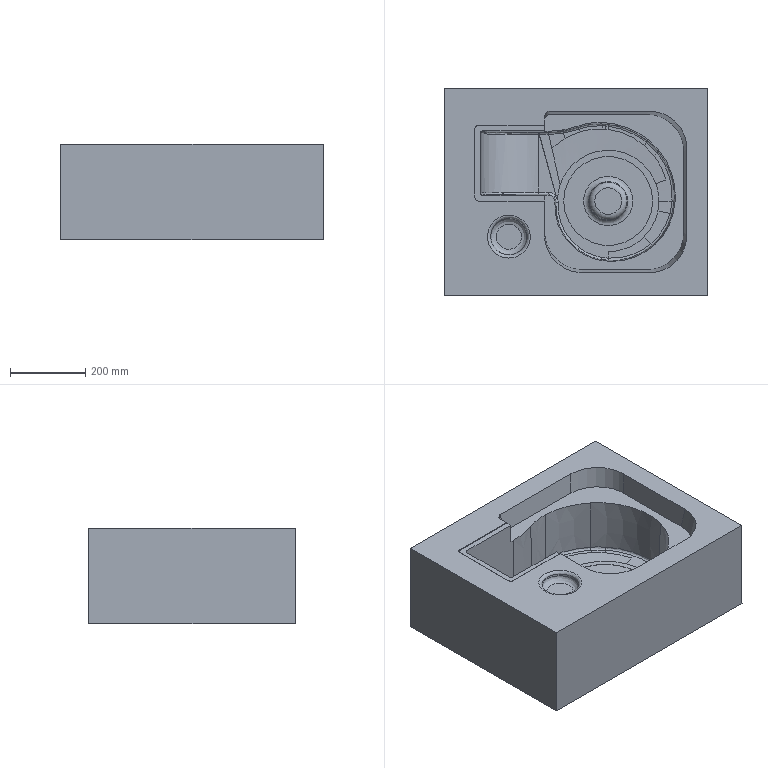NC program | NX | posted with a generic post | part box 700 x 550 x 255 mm
Lines 1 to 1065 of 43405:
N10 G17 G21 G94 G90
(CAVITY_MILL , TOOL : D50R6)
N12 T00 M6
N14 G54
N16 G17 G0 G90 X95.636 Y-22.406 S1000 M3
N18 G43 Z30. H0
N20 Z1.
N22 G94 G3 X120.189 Y0. Z-0.96 R22.5 F1800.
N24 G1 Y40.189
N26 X78.679
N28 G2 X90.983 Y-24.303 R174.834
N30 G1 Y-40.189
N32 X120.189
N34 Y0.
N36 X139.189
N38 Y59.189
N40 X47.771
N42 G2 X71.983 Y-24.299 R155.834
N44 G1 Y-59.189
N46 X139.189
N48 Y0.
N50 X158.189
N52 Y78.189
N54 X10.58
N56 G2 X8.765 Y76.49 R136.845
N58 X52.983 Y-24.295 R136.834
N60 G1 Y-78.189
N62 X158.189
N64 Y0.
N66 X177.189
N68 Y97.189
N70 X2.638
N72 G2 X-22.702 Y76.489 R117.845
N74 X33.983 Y-24.29 R117.834
N76 G1 Y-97.189
N78 X177.189
N80 Y0.
N82 X196.189
N84 Y116.159
N86 X196.19 Y116.19
N88 X196.154 Y116.189
N90 X-6.11
N92 G2 X-83.823 Y78.376 R98.845
N94 G1 X-171.096
N96 Y74.597
N98 X-83.796
N100 G2 X14.983 Y-24.286 R98.834
N102 G1 Y-114.246
N104 G3 X15.939 Y-116.171 R2.177
N106 X16.138 Y-116.189 R0.764
N108 G1 X196.007
N110 X196.083 Y-116.19
N112 X196.14 Y-116.188
N114 X196.189 Y-114.934
N116 Y0.
N118 X215.189
N120 Y116.025
N122 G3 X209.326 Y130.038 R19.039
N124 X196.022 Y135.189 R19.076
N126 G1 X-15.976
N128 G2 X-83.83 Y97.376 R79.845
N130 G1 X-190.096
N132 Y55.597
N134 X-83.807
N136 G2 X-4.017 Y-24.28 R79.834
N138 G1 Y-114.147
N140 G3 X7.641 Y-133.286 R21.177
N142 X16.17 Y-135.189 R19.764
N144 G1 X195.932
N146 G3 X205.75 Y-132.694 R19.944
N148 X215.074 Y-118.221 R18.797
N150 G1 X215.189 Y-115.309
N152 Y0.
N154 X234.189
N156 Y115.935
N158 G3 X222.394 Y143.831 R38.039
N160 X195.934 Y154.189 R38.076
N162 G1 X-27.545
N164 G2 X-83.838 Y116.376 R60.845
N166 G1 X-209.096
N168 Y36.597
N170 X-83.813
N172 G2 X-23.017 Y-24.274 R60.834
N174 G1 Y-114.079
N176 G3 X-0.698 Y-150.359 R40.177
N178 X16.191 Y-154.189 R38.764
N180 G1 X195.88
N182 G3 X215.095 Y-149.238 R38.944
N184 X234.042 Y-119.419 R37.797
N186 G1 X234.189 Y-115.684
N188 Y0.
N190 X253.189
N192 Y115.864
N194 G3 X235.462 Y157.623 R57.039
N196 X195.864 Y173.189 R57.076
N198 G1 X-42.212
N200 G2 X-83.846 Y135.376 R41.845
N202 G1 X-228.096
N204 Y17.597
N206 X-83.82
N208 G2 X-42.017 Y-24.268 R41.834
N210 G1 Y-114.023
N212 G3 X-9.039 Y-167.43 R59.177
N214 X16.208 Y-173.189 R57.764
N216 G1 X195.839
N218 G3 X224.438 Y-165.782 R57.944
N220 X253.013 Y-120.512 R56.797
N222 G1 X253.19 Y-116.031
N224 X253.189 Y-115.866
N226 Y0.
N228 X272.189
N230 Y115.802
N232 G3 X248.53 Y171.416 R76.039
N234 X195.804 Y192.189 R76.076
N236 G1 X-61.017
N238 Y177.233
N240 G2 X-83.851 Y154.376 R22.845
N242 G1 X-247.096
N244 Y-1.403
N246 X-83.829
N248 G2 X-61.017 Y-24.259 R22.834
N250 G1 Y-113.975
N252 G3 X-17.38 Y-184.502 R78.177
N254 X16.223 Y-192.189 R76.764
N256 G1 X195.804
N258 G3 X233.781 Y-182.326 R76.944
N260 X271.987 Y-121.551 R75.797
N262 G1 X272.193 Y-116.342
N264 X272.189 Y-115.802
N266 Y0.
N268 X247.189
N270 Z0.04
N272 G0 Z3.
N274 X94.586 Y-22.406
N276 Z0.04
N278 G3 X119.139 Y0. Z-1.92 R22.5
N280 G1 Y39.138
N282 X80.215
N284 G2 X92.034 Y-24.286 R175.897
N286 G1 Y-39.138
N288 X119.139
N290 Y0.
N292 X138.139
N294 Y58.138
N296 X49.662
N298 G2 X73.034 Y-24.284 R156.897
N300 G1 Y-58.138
N302 X138.139
N304 Y0.
N306 X157.139
N308 Y77.138
N310 X11.002
N312 G2 X10.308 Y76.485 R137.893
N314 X54.034 Y-24.281 R137.897
N316 G1 Y-77.138
N318 X157.139
N320 Y0.
N322 X176.139
N324 Y96.138
N326 X3.099
N328 G2 X-20.704 Y76.486 R118.893
N330 X35.034 Y-24.279 R118.897
N332 G1 Y-96.138
N334 X176.139
N336 Y0.
N338 X195.139
N340 Y115.138
N342 X-5.598
N344 G2 X-83.817 Y77.325 R99.893
N346 G1 X-170.045
N348 Y75.648
N350 X-83.83
N352 G2 X16.034 Y-24.276 R99.897
N354 G1 Y-114.18
N356 G3 X16.332 Y-115.138 R1.413
N358 G1 X195.139
N360 Y0.
N362 X214.139
N364 Y116.101
N366 G3 X208.285 Y129.568 R18.193
N368 X195.97 Y134.138 R18.328
N370 G1 X-15.391
N372 G2 X-83.825 Y96.325 R80.893
N374 G1 X-189.045
N376 Y56.648
N378 X-83.836
N380 G2 X-2.966 Y-24.272 R80.897
N382 G1 Y-114.102
N384 G3 X4.097 Y-129.712 R20.413
N386 X16.18 Y-134.138 R18.548
N388 G1 X195.985
N390 G3 X209.582 Y-128.269 R18.172
N392 X214.139 Y-116.061 R18.403
N394 G1 Y0.
N396 X233.139
N398 Y115.999
N400 G3 X221.006 Y143.681 R37.193
N402 X195.9 Y153.138 R37.328
N404 G1 X-26.842
N406 G2 X-83.833 Y115.325 R61.893
N408 G1 X-208.045
N410 Y37.648
N412 X-83.843
N414 G2 X-21.966 Y-24.268 R61.897
N416 G1 Y-114.049
N418 G3 X-8.276 Y-144.132 R39.413
N420 X16.2 Y-153.138 R37.548
N422 G1 X195.909
N424 G3 X223.723 Y-140.959 R37.172
N426 X233.139 Y-115.972 R37.403
N428 G1 Y0.
N430 X252.138
N432 Y115.897
N434 G3 X233.727 Y157.795 R56.193
N436 X195.845 Y172.138 R56.328
N438 G1 X-41.268
N440 G2 X-83.838 Y134.325 R42.893
N442 G1 X-227.045
N444 Y18.648
N446 X-83.849
N448 G2 X-40.966 Y-24.264 R42.897
N450 G1 Y-114.006
N452 G3 X-20.648 Y-158.551 R58.413
N454 X16.215 Y-172.138 R56.548
N456 G1 X195.849
N458 G3 X237.864 Y-153.649 R56.172
N460 X252.138 Y-115.884 R56.403
N462 G1 Y0.
N464 X271.138
N466 Y115.796
N468 G3 X246.448 Y171.908 R75.193
N470 X195.797 Y191.138 R75.328
N472 G1 X-59.966
N474 Y177.233
N476 G2 X-83.844 Y153.325 R23.893
N478 G1 X-246.045
N480 Y-0.352
N482 X-83.853
N484 G2 X-59.966 Y-24.259 R23.897
N486 G1 Y-113.97
N488 G3 X-33.021 Y-172.97 R77.413
N490 X16.229 Y-191.138 R75.548
N492 G1 X195.797
N494 G3 X252.006 Y-166.339 R75.172
N496 X271.138 Y-115.796 R75.403
N498 G1 Y0.
N500 X246.138
N502 Z-0.92
N504 G0 Z2.04
N506 X90.329 Y-21.815
N508 Z-0.92
N510 G3 X118.339 Y0. Z-3.064 R22.5
N512 G1 Y38.339
N514 X84.221
N516 G2 X90.318 Y5.39 R174.825
N518 X92.833 Y-24.019 R177.55
N520 G1 Y-38.339
N522 X118.339
N524 Y0.
N526 X137.339
N528 Y57.339
N530 X56.774
N532 G2 X71.455 Y2.967 R155.825
N534 X73.833 Y-24.04 R158.55
N536 G1 Y-57.339
N538 X137.339
N540 Y0.
N542 X156.339
N544 Y76.339
N546 X22.463
N548 G2 X52.587 Y0.545 R136.825
N550 X54.833 Y-24.063 R139.55
N552 G1 Y-76.339
N554 X156.339
N556 Y0.
N558 X175.339
N560 Y95.339
N562 X12.778
N564 G2 X-3.608 Y76.485 R117.82
N566 X33.712 Y-1.877 R117.825
N568 X35.833 Y-24.086 R120.55
N570 G1 Y-95.339
N572 X175.339
N574 Y0.
N576 X194.339
N578 Y114.339
N580 X2.3
N582 G2 X-35.662 Y76.485 R98.82
N584 X14.826 Y-4.298 R98.825
N586 X16.833 Y-24.112 R101.55
N588 G1 Y-114.19
N590 X16.832 Y-114.275
N592 X16.835 Y-114.339
N594 X194.339
N596 Y0.
N598 X213.339
N600 Y115.965
N602 G3 X209.454 Y127.18 R17.571
N604 X199.085 Y133.079 R16.832
N606 X196.656 Y133.339 R16.971
N608 G1 X-9.643
N610 G2 X-83.854 Y82.945 R79.82
N612 G1 X-174.712
N614 Y70.028
N616 X-83.848
N618 G2 X-4.081 Y-6.718 R79.825
N620 X-2.167 Y-24.141 R82.55
N622 G1 Y-114.106
N624 G3 X3.63 Y-128.196 R19.599
N626 X15.469 Y-133.344 R17.828
N628 G2 X16.205 Y-133.339 R57.
N630 G1 X196.641
N632 G3 X197.004 Y-133.315 R9.476
N634 G1 X197.206 Y-133.298
N636 G3 X207.952 Y-128.772 R17.207
N638 X213.209 Y-118.178 R17.016
N640 X213.339 Y-116.019 R14.176
N642 G1 Y0.
N644 X232.339
N646 Y115.897
N648 G3 X224.173 Y139.196 R36.571
N650 X202.242 Y151.815 R35.832
N652 X196.925 Y152.339 R35.971
N654 G1 X-23.921
N656 G2 X-83.851 Y101.945 R60.82
N658 G1 X-193.712
N660 Y51.028
N662 X-83.847
N664 G2 X-23.025 Y-9.135 R60.825
N666 X-21.167 Y-24.173 R63.55
N668 G1 Y-114.05
N670 G3 X-9.746 Y-141.69 R38.599
N672 X15.352 Y-152.349 R36.828
N674 G2 X16.205 Y-152.339 R38.
N676 G1 X196.971
N678 G3 X198.635 Y-152.245 R28.476
N680 X220.898 Y-142.678 R36.207
N682 X232.072 Y-120.462 R36.016
N684 X232.339 Y-115.927 R33.176
N686 G1 Y0.
N688 X251.339
N690 Y115.843
N692 G3 X238.892 Y151.211 R55.571
N694 X205.399 Y170.551 R54.832
N696 X197.128 Y171.339 R54.971
N698 G1 X-40.574
N700 G2 X-42.021 Y164.649 R44.309
N702 G1 Y162.755
N704 G2 X-83.849 Y120.945 R41.82
N706 G1 X-212.712
N708 Y32.028
N710 X-83.847
N712 G2 X-42.021 Y-9.797 R41.825
N714 G1 Y-11.67
N716 G2 X-40.167 Y-24.211 R44.55
N718 G1 Y-114.004
N720 G3 X-23.122 Y-155.183 R57.599
N722 X15.468 Y-171.354 R55.828
N724 G2 X16.205 Y-171.339 R19.
N726 G1 X197.2
N728 G3 X200.056 Y-171.192 R47.476
N730 X233.845 Y-156.585 R55.207
N732 X250.935 Y-122.743 R55.016
N734 X251.339 Y-115.857 R52.176
N736 G1 Y0.
N738 X270.339
N740 Y115.797
N742 G3 X253.61 Y163.226 R74.571
N744 X208.556 Y189.287 R73.832
N746 X195.855 Y190.349 R73.971
N748 G1 X195.794 Y190.339
N750 X-59.167
N752 Y177.233
N754 G2 X-61.021 Y167.824 R25.309
N756 G1 Y162.76
N758 G2 X-83.847 Y139.945 R22.82
N760 G1 X-231.712
N762 Y13.028
N764 X-83.847
N766 G2 X-61.021 Y-9.797 R22.825
N768 G1 Y-14.774
N770 Y-14.833
N772 G2 X-59.167 Y-24.259 R25.55
N774 G1 Y-113.965
N776 G3 X-36.497 Y-168.678 R76.599
N778 X16.169 Y-190.358 R74.828
N780 G1 X16.205 Y-190.339
N782 X195.794
N784 X195.855 Y-190.349
N786 G3 X201.604 Y-190.129 R66.476
N788 X246.792 Y-170.491 R74.207
N790 X269.797 Y-125.024 R74.016
N792 X270.339 Y-115.797 R71.176
N794 G1 Y0.
N796 X245.339
N798 Z-2.064
N800 G0 Z1.08
N802 X89.854 Y-21.814
N804 Z-2.064
N806 G3 X117.865 Y0. Z-4.208 R22.5
N808 G1 Y37.865
N810 X85.626
N812 G2 X92.091 Y-3.599 R176.047
N814 X93.307 Y-24.018 R178.341
N816 G1 Y-37.865
N818 X117.865
N820 Y0.
N822 X136.865
N824 Y56.865
N826 X58.35
N828 G2 X73.128 Y-5.044 R157.047
N830 X74.307 Y-24.039 R159.341
N832 G1 Y-56.865
N834 X136.865
N836 Y0.
N838 X155.865
N840 Y75.865
N842 X24.408
N844 G2 X54.161 Y-6.488 R138.047
N846 X55.307 Y-24.061 R140.341
N848 G1 Y-75.865
N850 X155.865
N852 Y0.
N854 X174.865
N856 Y94.865
N858 X13.938
N860 G2 X-1.824 Y76.484 R119.039
N862 X35.186 Y-7.931 R119.047
N864 X36.307 Y-24.085 R121.341
N866 G1 Y-94.865
N868 X174.865
N870 Y0.
N872 X193.865
N874 Y113.865
N876 X3.436
N878 G2 X-33.203 Y76.485 R100.039
N880 X16.199 Y-9.374 R100.047
N882 X17.307 Y-24.112 R102.341
N884 G1 Y-113.865
N886 X193.865
N888 Y0.
N890 X212.865
N892 Y116.035
N894 G3 X209.044 Y126.924 R17.054
N896 X198.295 Y132.72 R16.546
N898 X195.967 Y132.865 R16.134
N900 G1 X-8.516
N902 G2 X-83.845 Y81.723 R81.039
N904 G1 X-173.49
N906 Y71.25
N908 X-83.847
N910 G2 X-2.8 Y-9.796 R81.047
N912 G1 Y-10.853
N914 G2 X-1.693 Y-24.14 R83.341
N916 G1 Y-114.096
N918 G3 X4.32 Y-128.192 R19.125
N920 X16.158 Y-132.865 R17.173
N922 G1 X195.987
N924 G3 X207.209 Y-128.801 R16.994
N926 X212.591 Y-119.129 R16.462
N928 X212.865 Y-116.166 R16.163
N930 G1 Y0.
N932 X231.865
N934 Y115.89
N936 G3 X223.692 Y139.025 R36.054
N938 X200.672 Y151.571 R35.546
N940 X195.905 Y151.865 R35.134
N942 G1 X-22.764
N944 G2 X-83.843 Y100.723 R62.039
N946 G1 X-192.49
N948 Y52.25
N950 X-83.847
N952 G2 X-21.8 Y-9.797 R62.047
N954 G1 Y-12.508
N956 G2 X-20.693 Y-24.173 R64.341
N958 G1 Y-114.039
N960 G3 X-8.707 Y-142.024 R38.125
N962 X16.181 Y-151.865 R36.173
N964 G1 X195.918
N966 G3 X219.641 Y-143.17 R35.994
N968 X231.269 Y-122.613 R35.462
N970 X231.865 Y-116.166 R35.163
N972 G1 Y0.
N974 X250.865
N976 Y115.833
N978 G3 X238.341 Y151.125 R55.054
N980 X203.049 Y170.421 R54.546
N982 X195.857 Y170.865 R54.134
N984 G1 X-40.155
N986 G2 X-40.8 Y167.387 R44.764
N988 G1 Y162.757
N990 G2 X-83.842 Y119.723 R43.039
N992 G1 X-211.49
N994 Y33.25
N996 X-83.847
N998 G2 X-40.8 Y-9.797 R43.047
N1000 G1 Y-14.434
N1002 G2 X-39.693 Y-24.211 R45.341
N1004 G1 Y-113.993
N1006 G3 X-21.733 Y-155.855 R57.125
N1008 X16.198 Y-170.865 R55.173
N1010 G1 X195.863
N1012 G3 X232.072 Y-157.539 R54.994
N1014 X249.962 Y-126.011 R54.462
N1016 X250.865 Y-116.166 R54.163
N1018 G1 Y0.
N1020 X269.865
N1022 Y115.784
N1024 G3 X252.99 Y163.226 R74.054
N1026 X205.427 Y189.272 R73.546
N1028 X195.816 Y189.865 R73.134
N1030 G1 X-58.693
N1032 Y177.222
N1034 G2 X-59.8 Y169.81 R25.764
N1036 G1 Y162.759
N1038 G2 X-83.84 Y138.723 R24.039
N1040 G1 X-230.49
N1042 Y14.25
N1044 X-83.847
N1046 G2 X-59.8 Y-9.797 R24.047
N1048 G1 Y-16.836
N1050 G2 X-58.693 Y-24.259 R26.341
N1052 G1 Y-113.954
N1054 G3 X-34.759 Y-169.687 R76.125
N1056 X16.214 Y-189.865 R74.173
N1058 G1 X195.816
N1060 G3 X244.503 Y-171.908 R73.994
N1062 X268.504 Y-130.233 R73.462
N1064 G1 X268.646 Y-129.465
N1066 G3 X269.865 Y-116.166 R73.163
N1068 G1 Y0.
N1070 X244.865
N1072 Z-3.208
N1074 G0 Z-0.064
N1076 X89.62 Y-21.815
N1078 Z-3.208
N1080 G3 X117.63 Y0. Z-5.352 R22.5
N1082 G1 Y37.63
N1084 X86.454
N1086 G2 X91.667 Y11.256 R176.685
N1088 X92.938 Y-9.73 R173.807
N1090 X93.538 Y-24.069 R178.576
N1092 G1 Y-37.63
N1094 X117.63
N1096 Y0.
N1098 X136.63
N1100 Y56.63
N1102 X59.278
N1104 G2 X72.804 Y8.982 R157.685
N1106 X73.938 Y-9.886 R154.807
N1108 G1 Y-10.53
N1110 G2 X74.538 Y-24.085 R159.576
N1112 G1 Y-56.63
N1114 X136.63
N1116 Y0.
N1118 X155.63
N1120 Y75.63
N1122 X25.543
N1124 G2 X53.94 Y6.707 R138.685
N1126 X54.938 Y-9.876 R135.807
N1128 G1 Y-11.381
N1130 G2 X55.538 Y-24.102 R140.576
N1132 G1 Y-75.63
N1134 X155.63
N1136 Y0.
N1138 X174.63
N1140 Y94.63
N1142 X14.666
N1144 G2 X-0.754 Y76.496 R119.791
N1146 X35.077 Y4.432 R119.685
N1148 X35.938 Y-9.865 R116.807
N1150 G1 Y-12.291
N1152 G2 X36.538 Y-24.12 R121.576
N1154 G1 Y-94.63
N1156 X174.63
N1158 Y0.
N1160 X193.63
N1162 Y113.63
N1164 X4.144
N1166 G2 X-31.758 Y76.492 R100.791
N1168 X16.214 Y2.157 R100.685
N1170 X16.938 Y-9.853 R97.807
N1172 G1 Y-13.276
N1174 G2 X17.538 Y-24.14 R102.576
N1176 G1 Y-113.63
N1178 X193.63
N1180 Y0.
N1182 X212.63
N1184 Y115.9
N1186 G3 X210.822 Y123.75 R17.339
N1188 X199.982 Y132.164 R16.089
N1190 X196.005 Y132.63 R17.193
N1192 G1 X-7.82
N1194 G2 X-83.85 Y80.986 R81.791
N1196 G1 X-172.752
N1198 Y71.987
N1200 X-83.847
N1202 G2 X-81.174 Y71.925 R57.
N1204 X-2.65 Y-0.118 R81.685
N1206 X-2.062 Y-9.84 R78.807
N1208 G1 Y-14.358
N1210 G2 X-1.462 Y-24.162 R83.576
N1212 G1 Y-114.082
N1214 G3 X3.387 Y-126.926 R19.029
N1216 X15.752 Y-132.63 R17.178
N1218 G1 X195.919
N1220 G3 X206.809 Y-128.798 R16.826
N1222 X212.429 Y-118.644 R16.323
N1224 X212.63 Y-115.839 R18.672
N1226 G1 Y0.
N1228 X231.63
N1230 Y115.85
N1232 G3 X227.8 Y132.279 R36.339
N1234 X204.25 Y150.679 R35.089
N1236 X196.005 Y151.63 R36.193
N1238 G1 X-22.059
N1240 G2 X-83.85 Y99.986 R62.791
N1242 G1 X-191.752
N1244 Y52.987
N1246 X-83.847
N1248 G2 X-81.926 Y52.939 R38.
N1250 X-21.513 Y-2.393 R62.685
N1252 X-21.062 Y-9.826 R59.807
N1254 G1 Y-15.572
N1256 G2 X-20.462 Y-24.186 R64.576
N1258 G1 Y-114.03
N1260 G3 X-10.764 Y-139.605 R38.029
N1262 X15.561 Y-151.63 R36.178
N1264 G1 X195.848
N1266 G3 X218.978 Y-143.39 R35.826
N1268 X231.238 Y-121.335 R35.323
N1270 X231.63 Y-115.814 R37.672
N1272 G1 Y0.
N1274 X250.63
N1276 Y115.811
N1278 G3 X244.779 Y140.806 R55.339
N1280 X208.518 Y169.193 R54.089
N1282 X196.005 Y170.63 R55.193
N1284 G1 X-39.953
N1286 G2 X-40.062 Y169.935 R44.995
N1288 G1 Y162.737
N1290 G2 X-83.851 Y118.986 R43.791
N1292 G1 X-210.752
N1294 Y33.987
N1296 X-83.847
N1298 G2 X-82.702 Y33.953 R19.
N1300 X-40.376 Y-4.669 R43.685
N1302 X-40.062 Y-9.808 R40.807
N1304 G1 Y-16.984
N1306 G2 X-39.462 Y-24.215 R45.576
N1308 G1 Y-113.989
N1310 G3 X-24.915 Y-152.283 R57.029
N1312 X15.416 Y-170.63 R55.178
N1314 G1 X195.791
N1316 G3 X231.147 Y-157.982 R54.826
N1318 X250.043 Y-124.047 R54.323
N1320 X250.63 Y-115.795 R56.672
N1322 G1 Y0.
N1324 X269.63
N1326 Y115.778
N1328 G3 X261.758 Y149.334 R74.339
N1330 X213.524 Y187.536 R73.089
N1332 G1 X212.826 Y187.698
N1334 G3 X196.005 Y189.63 R74.193
N1336 G1 X-58.462
N1338 Y177.222
N1340 G2 X-59.062 Y171.706 R25.996
N1342 G1 Y162.748
N1344 G2 X-83.852 Y137.986 R24.791
N1346 G1 X-229.752
N1348 Y14.987
N1350 X-83.847
N1352 X-83.804 Y14.966
N1354 G2 X-59.24 Y-6.946 R24.685
N1356 X-59.062 Y-9.786 R21.807
N1358 G1 Y-18.739
N1360 G2 X-58.462 Y-24.252 R26.576
N1362 G1 Y-113.954
N1364 G3 X-39.066 Y-164.962 R76.029
N1366 X16.182 Y-189.635 R74.178
N1368 G1 X16.218 Y-189.63
N1370 X195.743
N1372 G3 X243.316 Y-172.574 R73.826
N1374 X268.849 Y-126.76 R73.323
N1376 X269.63 Y-115.778 R75.672
N1378 G1 Y0.
N1380 X244.63
N1382 Z-4.352
N1384 G0 Z-1.208
N1386 X89.459 Y-21.815
N1388 Z-4.352
N1390 G3 X117.469 Y0. Z-6.496 R22.5
N1392 G1 Y37.469
N1394 X86.957
N1396 G2 X93.374 Y-9.73 R177.21
N1398 G1 Y-15.784
N1400 G2 X93.576 Y-23.943 R181.712
N1402 G1 Y-37.469
N1404 X117.469
N1406 Y0.
N1408 X136.469
N1410 Y56.469
N1412 X59.832
N1414 G2 X74.374 Y-9.736 R158.21
N1416 G1 Y-16.245
N1418 G2 X74.576 Y-23.966 R162.712
N1420 G1 Y-56.469
N1422 X136.469
N1424 Y0.
N1426 X155.469
N1428 Y75.469
N1430 X26.213
N1432 G2 X55.374 Y-9.742 R139.21
N1434 G1 Y-16.735
N1436 G2 X55.576 Y-23.991 R143.712
N1438 G1 Y-75.469
N1440 X155.469
N1442 Y0.
N1444 X174.469
N1446 Y94.469
N1448 X15.099
N1450 G2 X-0.122 Y76.483 R120.196
N1452 X36.374 Y-9.748 R120.21
N1454 G1 Y-17.258
N1456 G2 X36.576 Y-24.018 R124.712
N1458 G1 Y-94.469
N1460 X174.469
N1462 Y0.
N1464 X193.469
N1466 Y113.469
N1468 X4.566
N1470 G2 X-30.913 Y76.483 R101.196
N1472 X17.374 Y-9.755 R101.21
N1474 G1 Y-17.823
N1476 G2 X17.576 Y-24.047 R105.712
N1478 G1 Y-113.469
N1480 X193.469
N1482 Y0.
N1484 X212.469
N1486 Y115.732
N1488 G3 X207.95 Y127.417 R16.798
N1490 X197.329 Y132.399 R16.53
N1492 X195.485 Y132.469 R25.423
N1494 G1 X-7.406
N1496 G2 X-83.844 Y80.55 R82.196
N1498 G1 X-172.317
N1500 Y72.423
N1502 X-83.858
N1504 G2 X-1.626 Y-9.761 R82.21
N1506 G1 Y-18.441
N1508 G2 X-1.424 Y-24.079 R86.712
N1510 G1 Y-113.923
N1512 G3 X4.257 Y-127.637 R18.859
N1514 X16.181 Y-132.469 R17.019
N1516 G1 X195.713
N1518 G3 X206.678 Y-128.609 R16.892
N1520 X212.4 Y-117.333 R16.44
N1522 X212.469 Y-115.49 R25.879
N1524 G1 Y0.
N1526 X231.469
N1528 Y115.653
N1530 G3 X221.718 Y140.511 R35.798
N1532 X198.755 Y151.346 R35.53
N1534 X195.499 Y151.469 R44.423
N1536 G1 X-21.64
N1538 G2 X-83.84 Y99.55 R63.196
N1540 G1 X-191.317
N1542 Y53.423
N1544 X-83.855
N1546 G2 X-20.626 Y-9.767 R63.21
N1548 G1 Y-19.131
N1550 G2 X-20.424 Y-24.115 R67.712
N1552 G1 Y-113.848
N1554 G3 X-9.012 Y-141.236 R37.859
N1556 X16.197 Y-151.469 R36.019
N1558 G1 X195.634
N1560 G3 X218.891 Y-143.165 R35.892
N1562 X231.347 Y-118.739 R35.44
N1564 X231.469 Y-115.509 R44.879
N1566 G1 Y0.
N1568 X250.469
N1570 Y115.59
N1572 G3 X235.486 Y153.605 R54.798
N1574 X200.18 Y170.292 R54.53
N1576 X195.51 Y170.469 R63.423
N1578 G1 X-39.626
N1580 Y162.733
N1582 G2 X-83.836 Y118.55 R44.196
N1584 G1 X-210.317
N1586 Y34.423
N1588 X-83.851
N1590 G2 X-39.626 Y-9.773 R44.21
N1592 G1 Y-19.928
N1594 G2 X-39.424 Y-24.157 R48.712
N1596 G1 Y-113.788
N1598 G3 X-22.281 Y-154.836 R56.859
N1600 X16.21 Y-170.469 R55.019
N1602 G1 X195.573
N1604 G3 X231.104 Y-157.72 R54.892
N1606 X250.295 Y-120.145 R54.44
N1608 X250.469 Y-115.523 R63.879
N1610 G1 Y0.
N1612 X269.469
N1614 Y115.536
N1616 G3 X249.254 Y166.698 R73.798
N1618 X201.604 Y189.239 R73.53
N1620 X195.52 Y189.469 R82.423
N1622 G1 X-58.424
N1624 Y177.182
N1626 G2 X-58.626 Y173.967 R25.901
N1628 G1 Y162.737
N1630 G2 X-83.832 Y137.55 R25.196
N1632 G1 X-229.317
N1634 Y15.423
N1636 X-83.847
N1638 G2 X-58.626 Y-9.777 R25.21
N1640 G1 Y-20.903
N1642 G2 X-58.424 Y-24.209 R29.712
N1644 G1 Y-113.737
N1646 G3 X-35.549 Y-168.435 R75.859
N1648 X16.221 Y-189.469 R74.019
N1650 G1 X195.52
N1652 G3 X243.316 Y-172.276 R73.892
N1654 X269.243 Y-121.551 R73.44
N1656 X269.469 Y-115.536 R82.879
N1658 G1 Y0.
N1660 X244.469
N1662 Z-5.496
N1664 G0 Z-2.352
N1666 X89.299 Y-21.814
N1668 Z-5.496
N1670 G3 X117.309 Y0.001 Z-7.64 R22.5
N1672 G1 Y37.309
N1674 X87.207
N1676 G2 X93.572 Y-9.717 R177.406
N1678 G1 X93.576 Y-37.309
N1680 X117.309
N1682 Y0.001
N1684 X136.309 Y0.
N1686 Y56.309
N1688 X60.124
N1690 G2 X74.572 Y-9.724 R158.406
N1692 G1 X74.578 Y-56.309
N1694 X136.309
N1696 Y0.
N1698 X155.309
N1700 Y75.309
N1702 X26.588
N1704 G2 X55.572 Y-9.731 R139.406
N1706 G1 X55.581 Y-75.309
N1708 X155.309
N1710 Y0.
N1712 X174.309
N1714 Y94.309
N1716 X15.22
N1718 G2 X0.157 Y76.488 R120.412
N1720 X36.572 Y-9.739 R120.406
N1722 G1 X36.584 Y-94.309
N1724 X174.309
N1726 Y0.
N1728 X193.309
N1730 Y113.309
N1732 X4.695
N1734 G2 X-30.541 Y76.488 R101.412
N1736 X17.572 Y-9.746 R101.406
N1738 G1 X17.586 Y-113.309
N1740 X193.309
N1742 Y0.
N1744 X212.309
N1746 Y115.653
N1748 G3 X208.735 Y126.165 R16.978
N1750 X198.043 Y132.143 R16.308
N1752 X195.379 Y132.309 R22.005
N1754 G1 X-7.262
N1756 G2 X-83.803 Y80.352 R82.412
N1758 G1 X-172.119
N1760 Y72.621
N1762 X-83.859
N1764 G2 X-1.428 Y-9.753 R82.406
N1766 G1 X-1.414 Y-113.89
N1768 G3 X2.845 Y-125.934 R19.161
N1770 X16.209 Y-132.309 R17.161
N1772 G1 X195.568
N1774 G3 X206.183 Y-128.72 R16.977
N1776 X212.145 Y-118.024 R16.321
N1778 X212.309 Y-115.356 R21.839
N1780 G1 Y0.
N1782 X231.309
N1784 Y115.55
N1786 G3 X223.647 Y137.94 R35.978
N1788 X200.389 Y150.997 R35.308
N1790 X195.392 Y151.309 R41.005
N1792 G1 X-21.472
N1794 G2 X-83.812 Y99.352 R63.412
N1796 G1 X-191.119
N1798 Y53.621
N1800 X-83.855
N1802 G2 X-20.428 Y-9.761 R63.406
N1804 G1 X-20.414 Y-113.89
N1806 G3 X-11.933 Y-137.877 R38.161
N1808 X16.215 Y-151.309 R36.161
N1810 G1 X195.504
N1812 G3 X217.982 Y-143.613 R35.977
N1814 X231.002 Y-120.358 R35.321
N1816 X231.309 Y-115.352 R40.839
N1818 G1 Y0.
N1820 X250.309
N1822 Y115.448
N1824 G3 X238.559 Y149.715 R54.978
N1826 X202.735 Y169.852 R54.308
N1828 X195.403 Y170.309 R60.005
N1830 G1 X-39.428
N1832 Y162.787
N1834 G2 X-83.817 Y118.352 R44.412
N1836 G1 X-210.119
N1838 Y34.621
N1840 X-83.852
N1842 G2 X-39.428 Y-9.768 R44.406
N1844 G1 Y-23.158
N1846 X-39.414 Y-24.041
N1848 Y-113.89
N1850 G3 X-26.71 Y-149.819 R57.161
N1852 X16.22 Y-170.309 R55.161
N1854 G1 X195.454
N1856 G3 X229.78 Y-158.507 R54.977
N1858 X249.858 Y-122.691 R54.321
N1860 X250.309 Y-115.349 R59.839
N1862 G1 Y0.
N1864 X269.309
N1866 Y115.346
N1868 G3 X253.471 Y161.489 R73.978
N1870 X205.08 Y188.706 R73.308
N1872 X195.412 Y189.309 R79.005
N1874 G1 X-58.414
N1876 Y177.172
N1878 X-58.428 Y176.285
N1880 Y162.781
N1882 G2 X-83.823 Y137.352 R25.412
N1884 G1 X-229.119
N1886 Y15.621
N1888 X-83.847
N1890 G2 X-58.428 Y-9.773 R25.406
N1892 G1 Y-23.315
N1894 X-58.414 Y-24.199
N1896 Y-113.89
N1898 G3 X-41.488 Y-161.762 R76.161
N1900 X16.224 Y-189.309 R74.161
N1902 G1 X195.412
N1904 G3 X241.578 Y-173.4 R73.977
N1906 X268.714 Y-125.024 R73.321
N1908 X269.309 Y-115.346 R78.839
N1910 G1 Y0.
N1912 X244.309
N1914 Z-6.64
N1916 G0 Z-3.496
N1918 X89.137 Y-21.815
N1920 Z-6.64
N1922 G3 X117.148 Y0. Z-8.784 R22.5
N1924 G1 Y37.148
N1926 X87.286
N1928 G2 X93.596 Y-9.75 R177.4
N1930 G1 Y-37.148
N1932 X117.148
N1934 Y0.
N1936 X136.148
N1938 Y56.148
N1940 X60.239
N1942 G2 X74.596 Y-9.75 R158.4
N1944 G1 Y-56.148
N1946 X136.148
N1948 Y0.
N1950 X155.148
N1952 Y75.148
N1954 X26.764
N1956 G2 X55.596 Y-9.75 R139.4
N1958 G1 Y-75.148
N1960 X155.148
N1962 Y0.
N1964 X174.148
N1966 Y94.148
N1968 X15.161
N1970 G2 X0.219 Y76.486 R120.4
N1972 X36.596 Y-9.749 R120.4
N1974 G1 Y-94.148
N1976 X174.148
N1978 Y0.
N1980 X193.148
N1982 Y113.148
N1984 X4.653
N1986 G2 X-30.459 Y76.486 R101.4
N1988 X17.596 Y-9.749 R101.4
N1990 G1 Y-113.148
N1992 X193.148 Y-113.149
N1994 Y0.
N1996 X212.148
N1998 Y115.362
N2000 G3 X209.107 Y125.295 R17.132
N2002 X199.218 Y131.742 R16.108
N2004 X195.257 Y132.148 R18.592
N2006 G1 X-7.285
N2008 G2 X-83.802 Y80.321 R82.4
N2010 G1 X-172.088
N2012 Y72.652
N2014 X-83.802
N2016 G2 X-1.404 Y-9.749 R82.4
N2018 G1 Y-113.718
N2020 G3 X2.515 Y-125.35 R19.22
N2022 X16.225 Y-132.148 R17.218
N2024 G1 X195.46 Y-132.149
N2026 G3 X205.307 Y-129.098 R17.142
N2028 X211.916 Y-118.295 R16.208
N2030 X212.148 Y-115.218 R20.246
N2032 G1 Y0.
N2034 X231.148
N2036 Y115.296
N2038 G3 X224.664 Y136.203 R36.132
N2040 X203.106 Y150.34 R35.108
N2042 X195.224 Y151.148 R37.592
N2044 G1 X-21.469
N2046 G2 X-83.802 Y99.321 R63.4
N2048 G1 X-191.088
N2050 Y53.652
N2052 X-83.802
N2054 G2 X-20.404 Y-9.748 R63.4
N2056 G1 Y-113.718
N2058 G3 X-12.611 Y-136.848 R38.22
N2060 X16.227 Y-151.148 R36.218
N2062 G1 X195.365
N2064 G3 X216.239 Y-144.638 R36.142
N2066 X230.704 Y-121.128 R35.208
N2068 X231.148 Y-115.21 R39.246
N2070 G1 Y0.
N2072 X250.148
N2074 Y115.243
N2076 G3 X240.222 Y147.11 R55.132
N2078 X206.994 Y168.938 R54.108
N2080 X195.198 Y170.148 R56.592
N2082 G1 X-39.404
N2084 Y162.721
N2086 G2 X-83.803 Y118.321 R44.4
N2088 G1 X-210.088
N2090 Y34.652
N2092 X-83.803
N2094 G2 X-39.404 Y-9.748 R44.4
N2096 G1 Y-113.718
N2098 G3 X-27.737 Y-148.346 R57.22
N2100 X16.23 Y-170.148 R55.218
N2102 G1 X195.271
N2104 G3 X227.17 Y-160.179 R55.142
N2106 X249.494 Y-123.944 R54.208
N2108 X250.148 Y-115.203 R58.246
N2110 G1 Y0.
N2112 X269.148
N2114 Y115.198
N2116 G3 X255.78 Y158.016 R74.132
N2118 X210.882 Y187.536 R73.108
N2120 X195.176 Y189.148 R75.592
N2122 G1 X-58.404
N2124 Y162.721
N2126 G2 X-83.803 Y137.321 R25.4
N2128 G1 X-229.088